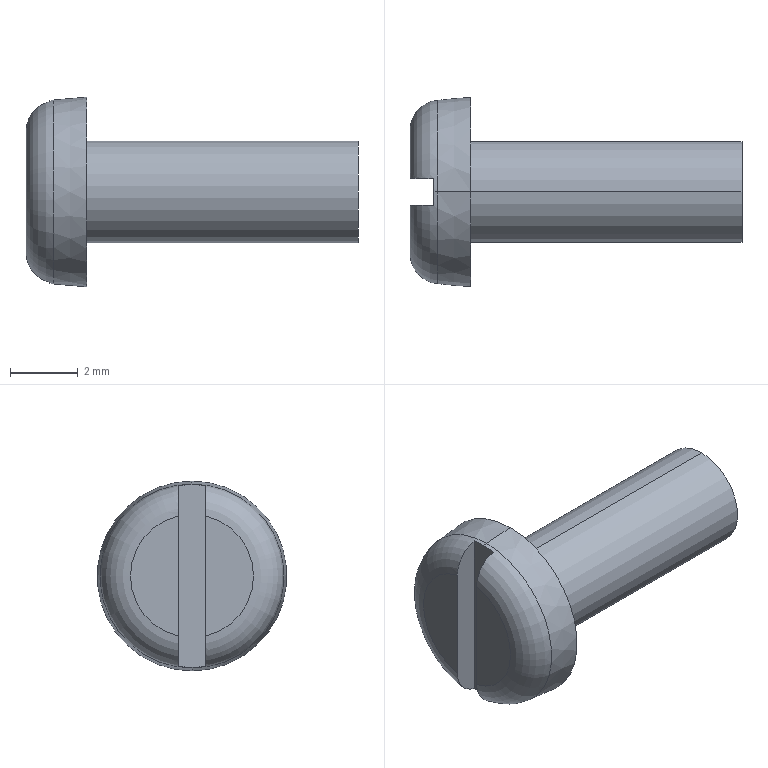Part | SolidWorks | features Fillet 2, Attribute 1, Cut 1, LPattern 1, RevCut 1, Revolution 1 | 1 solid | 13 faces | box 9.8 x 5.6 x 5.6 mm | volume 93.48 mm3 | plane 7 | torus 2 | cone 2 | cylinder 2 | commonest cylinder face diameters 3 x2
STEP:
#1=CARTESIAN_POINT('',(0.8216,0.,-2.714));
#2=VERTEX_POINT('',#1);
#3=CARTESIAN_POINT('',(0.8216,0.,2.714));
#4=VERTEX_POINT('',#3);
#5=CARTESIAN_POINT('',(0.8216,0.,0.));
#6=DIRECTION('',(1.,0.,0.));
#7=DIRECTION('',(0.,0.,1.));
#8=AXIS2_PLACEMENT_3D('',#5,#6,#7);
#9=CIRCLE('',#8,2.714);
#10=EDGE_CURVE('',#2,#4,#9,.T.);
#11=ORIENTED_EDGE('',*,*,#10,.F.);
#12=CARTESIAN_POINT('',(0.7,0.,-2.695));
#13=VERTEX_POINT('',#12);
#14=CARTESIAN_POINT('',(0.9,0.,-1.818));
#15=DIRECTION('',(0.,1.,0.));
#16=DIRECTION('',(0.,0.,1.));
#17=AXIS2_PLACEMENT_3D('',#14,#15,#16);
#18=CIRCLE('',#17,0.9);
#19=EDGE_CURVE('',#2,#13,#18,.T.);
#20=ORIENTED_EDGE('',*,*,#19,.T.);
#21=CARTESIAN_POINT('',(0.7,0.4,-2.665));
#22=VERTEX_POINT('',#21);
#23=CARTESIAN_POINT('',(0.7,0.,0.));
#24=DIRECTION('',(1.,0.,0.));
#25=DIRECTION('',(0.,0.,1.));
#26=AXIS2_PLACEMENT_3D('',#23,#24,#25);
#27=CIRCLE('',#26,2.695);
#28=EDGE_CURVE('',#13,#22,#27,.T.);
#29=ORIENTED_EDGE('',*,*,#28,.T.);
#30=CARTESIAN_POINT('',(0.,0.4,-1.773));
#31=VERTEX_POINT('',#30);
#32=CARTESIAN_POINT('',(0.,0.4,-1.773));
#33=CARTESIAN_POINT('',(0.,0.4,-1.977));
#34=CARTESIAN_POINT('',(0.06786,0.4,-2.18));
#35=CARTESIAN_POINT('',(0.3198,0.4,-2.504));
#36=CARTESIAN_POINT('',(0.5021,0.4,-2.62));
#37=CARTESIAN_POINT('',(0.7,0.4,-2.665));
#38=B_SPLINE_CURVE_WITH_KNOTS('',3,(#32,#33,#34,#35,#36,#37),.UNSPECIFIED.,.F.,.F.,(4,2,4),(0.004973,0.005582,0.006191),.UNSPECIFIED.);
#39=EDGE_CURVE('',#31,#22,#38,.T.);
#40=ORIENTED_EDGE('',*,*,#39,.F.);
#41=CARTESIAN_POINT('',(0.,0.4,1.773));
#42=VERTEX_POINT('',#41);
#43=CARTESIAN_POINT('',(0.,0.,0.));
#44=DIRECTION('',(-1.,0.,0.));
#45=DIRECTION('',(0.,0.,1.));
#46=AXIS2_PLACEMENT_3D('',#43,#44,#45);
#47=CIRCLE('',#46,1.818);
#48=EDGE_CURVE('',#42,#31,#47,.T.);
#49=ORIENTED_EDGE('',*,*,#48,.F.);
#50=CARTESIAN_POINT('',(0.7,0.4,2.665));
#51=VERTEX_POINT('',#50);
#52=CARTESIAN_POINT('',(0.7,0.4,2.665));
#53=CARTESIAN_POINT('',(0.4997,0.4,2.619));
#54=CARTESIAN_POINT('',(0.3202,0.4,2.504));
#55=CARTESIAN_POINT('',(0.06789,0.4,2.18));
#56=CARTESIAN_POINT('',(0.,0.4,1.978));
#57=CARTESIAN_POINT('',(0.,0.4,1.773));
#58=B_SPLINE_CURVE_WITH_KNOTS('',3,(#52,#53,#54,#55,#56,#57),.UNSPECIFIED.,.F.,.F.,(4,2,4),(0.00365,0.004259,0.004869),.UNSPECIFIED.);
#59=EDGE_CURVE('',#51,#42,#58,.T.);
#60=ORIENTED_EDGE('',*,*,#59,.F.);
#61=CARTESIAN_POINT('',(0.7,0.,2.695));
#62=VERTEX_POINT('',#61);
#63=CARTESIAN_POINT('',(0.7,0.,0.));
#64=DIRECTION('',(1.,0.,0.));
#65=DIRECTION('',(0.,0.,1.));
#66=AXIS2_PLACEMENT_3D('',#63,#64,#65);
#67=CIRCLE('',#66,2.695);
#68=EDGE_CURVE('',#51,#62,#67,.T.);
#69=ORIENTED_EDGE('',*,*,#68,.T.);
#70=CARTESIAN_POINT('',(0.9,0.,1.818));
#71=DIRECTION('',(0.,-1.,0.));
#72=DIRECTION('',(0.,0.,-1.));
#73=AXIS2_PLACEMENT_3D('',#70,#71,#72);
#74=CIRCLE('',#73,0.9);
#75=EDGE_CURVE('',#4,#62,#74,.T.);
#76=ORIENTED_EDGE('',*,*,#75,.F.);
#77=EDGE_LOOP('',(#11,#20,#29,#40,#49,#60,#69,#76));
#78=FACE_OUTER_BOUND('',#77,.T.);
#79=CARTESIAN_POINT('',(0.9,0.,0.));
#80=DIRECTION('',(-1.,0.,0.));
#81=DIRECTION('',(0.,0.,1.));
#82=AXIS2_PLACEMENT_3D('',#79,#80,#81);
#83=TOROIDAL_SURFACE('',#82,1.818,0.9);
#84=ADVANCED_FACE('',(#78),#83,.T.);
#85=ORIENTED_EDGE('',*,*,#10,.T.);
#86=CARTESIAN_POINT('',(1.8,0.,2.8));
#87=VERTEX_POINT('',#86);
#88=CARTESIAN_POINT('',(0.,0.,2.643));
#89=DIRECTION('',(0.9962,0.,0.08716));
#90=VECTOR('',#89,1000.);
#91=LINE('',#88,#90);
#92=EDGE_CURVE('',#4,#87,#91,.T.);
#93=ORIENTED_EDGE('',*,*,#92,.T.);
#94=CARTESIAN_POINT('',(1.8,0.,-2.8));
#95=VERTEX_POINT('',#94);
#96=CARTESIAN_POINT('',(1.8,0.,0.));
#97=DIRECTION('',(-1.,0.,0.));
#98=DIRECTION('',(0.,0.,1.));
#99=AXIS2_PLACEMENT_3D('',#96,#97,#98);
#100=CIRCLE('',#99,2.8);
#101=EDGE_CURVE('',#87,#95,#100,.T.);
#102=ORIENTED_EDGE('',*,*,#101,.T.);
#103=CARTESIAN_POINT('',(0.,0.,-2.643));
#104=DIRECTION('',(0.9962,0.,-0.08716));
#105=VECTOR('',#104,1000.);
#106=LINE('',#103,#105);
#107=EDGE_CURVE('',#2,#95,#106,.T.);
#108=ORIENTED_EDGE('',*,*,#107,.F.);
#109=EDGE_LOOP('',(#85,#93,#102,#108));
#110=FACE_OUTER_BOUND('',#109,.T.);
#111=CARTESIAN_POINT('',(0.,0.,0.));
#112=DIRECTION('',(1.,0.,0.));
#113=DIRECTION('',(0.,0.,-1.));
#114=AXIS2_PLACEMENT_3D('',#111,#112,#113);
#115=CONICAL_SURFACE('',#114,2.643,0.08727);
#116=ADVANCED_FACE('',(#110),#115,.T.);
#117=CARTESIAN_POINT('',(9.8,0.,1.5));
#118=VERTEX_POINT('',#117);
#119=CARTESIAN_POINT('',(9.8,0.,-1.5));
#120=VERTEX_POINT('',#119);
#121=CARTESIAN_POINT('',(9.8,0.,0.));
#122=DIRECTION('',(-1.,0.,0.));
#123=DIRECTION('',(0.,0.,1.));
#124=AXIS2_PLACEMENT_3D('',#121,#122,#123);
#125=CIRCLE('',#124,1.5);
#126=EDGE_CURVE('',#118,#120,#125,.T.);
#127=ORIENTED_EDGE('',*,*,#126,.T.);
#128=CARTESIAN_POINT('',(1.8,0.,-1.5));
#129=VERTEX_POINT('',#128);
#130=CARTESIAN_POINT('',(-25.4,0.,-1.5));
#131=DIRECTION('',(-1.,0.,0.));
#132=VECTOR('',#131,1000.);
#133=LINE('',#130,#132);
#134=EDGE_CURVE('',#120,#129,#133,.T.);
#135=ORIENTED_EDGE('',*,*,#134,.T.);
#136=CARTESIAN_POINT('',(1.8,0.,1.5));
#137=VERTEX_POINT('',#136);
#138=CARTESIAN_POINT('',(1.8,0.,0.));
#139=DIRECTION('',(-1.,0.,0.));
#140=DIRECTION('',(0.,0.,1.));
#141=AXIS2_PLACEMENT_3D('',#138,#139,#140);
#142=CIRCLE('',#141,1.5);
#143=EDGE_CURVE('',#137,#129,#142,.T.);
#144=ORIENTED_EDGE('',*,*,#143,.F.);
#145=CARTESIAN_POINT('',(-25.4,0.,1.5));
#146=DIRECTION('',(-1.,0.,0.));
#147=VECTOR('',#146,1000.);
#148=LINE('',#145,#147);
#149=EDGE_CURVE('',#118,#137,#148,.T.);
#150=ORIENTED_EDGE('',*,*,#149,.F.);
#151=EDGE_LOOP('',(#127,#135,#144,#150));
#152=FACE_OUTER_BOUND('',#151,.T.);
#153=CARTESIAN_POINT('',(-25.4,0.,0.));
#154=DIRECTION('',(-1.,0.,0.));
#155=DIRECTION('',(0.,0.,1.));
#156=AXIS2_PLACEMENT_3D('',#153,#154,#155);
#157=CYLINDRICAL_SURFACE('',#156,1.5);
#158=ADVANCED_FACE('',(#152),#157,.T.);
#159=CARTESIAN_POINT('',(0.,0.4,2.8));
#160=DIRECTION('',(0.,0.,-1.));
#161=VECTOR('',#160,1000.);
#162=LINE('',#159,#161);
#163=EDGE_CURVE('',#42,#31,#162,.T.);
#164=ORIENTED_EDGE('',*,*,#163,.F.);
#165=ORIENTED_EDGE('',*,*,#48,.T.);
#166=EDGE_LOOP('',(#164,#165));
#167=FACE_OUTER_BOUND('',#166,.T.);
#168=CARTESIAN_POINT('',(0.,0.,0.));
#169=DIRECTION('',(-1.,0.,0.));
#170=DIRECTION('',(0.,0.,1.));
#171=AXIS2_PLACEMENT_3D('',#168,#169,#170);
#172=PLANE('',#171);
#173=ADVANCED_FACE('',(#167),#172,.T.);
#174=ORIENTED_EDGE('',*,*,#134,.F.);
#175=CARTESIAN_POINT('',(9.8,0.,0.));
#176=DIRECTION('',(-1.,0.,0.));
#177=DIRECTION('',(0.,0.,1.));
#178=AXIS2_PLACEMENT_3D('',#175,#176,#177);
#179=CIRCLE('',#178,1.5);
#180=EDGE_CURVE('',#120,#118,#179,.T.);
#181=ORIENTED_EDGE('',*,*,#180,.T.);
#182=ORIENTED_EDGE('',*,*,#149,.T.);
#183=CARTESIAN_POINT('',(1.8,0.,0.));
#184=DIRECTION('',(-1.,0.,0.));
#185=DIRECTION('',(0.,0.,1.));
#186=AXIS2_PLACEMENT_3D('',#183,#184,#185);
#187=CIRCLE('',#186,1.5);
#188=EDGE_CURVE('',#129,#137,#187,.T.);
#189=ORIENTED_EDGE('',*,*,#188,.F.);
#190=EDGE_LOOP('',(#174,#181,#182,#189));
#191=FACE_OUTER_BOUND('',#190,.T.);
#192=CARTESIAN_POINT('',(-25.4,0.,0.));
#193=DIRECTION('',(-1.,0.,0.));
#194=DIRECTION('',(0.,0.,1.));
#195=AXIS2_PLACEMENT_3D('',#192,#193,#194);
#196=CYLINDRICAL_SURFACE('',#195,1.5);
#197=ADVANCED_FACE('',(#191),#196,.T.);
#198=ORIENTED_EDGE('',*,*,#126,.F.);
#199=ORIENTED_EDGE('',*,*,#180,.F.);
#200=EDGE_LOOP('',(#198,#199));
#201=FACE_OUTER_BOUND('',#200,.T.);
#202=CARTESIAN_POINT('',(9.8,1.5,0.));
#203=DIRECTION('',(1.,0.,0.));
#204=DIRECTION('',(0.,0.,-1.));
#205=AXIS2_PLACEMENT_3D('',#202,#203,#204);
#206=PLANE('',#205);
#207=ADVANCED_FACE('',(#201),#206,.T.);
#208=CARTESIAN_POINT('',(0.,-0.4,-1.773));
#209=VERTEX_POINT('',#208);
#210=CARTESIAN_POINT('',(0.,-0.4,1.773));
#211=VERTEX_POINT('',#210);
#212=CARTESIAN_POINT('',(0.,-0.4,-2.8));
#213=DIRECTION('',(0.,0.,1.));
#214=VECTOR('',#213,1000.);
#215=LINE('',#212,#214);
#216=EDGE_CURVE('',#209,#211,#215,.T.);
#217=ORIENTED_EDGE('',*,*,#216,.F.);
#218=CARTESIAN_POINT('',(0.,0.,0.));
#219=DIRECTION('',(-1.,0.,0.));
#220=DIRECTION('',(0.,0.,1.));
#221=AXIS2_PLACEMENT_3D('',#218,#219,#220);
#222=CIRCLE('',#221,1.818);
#223=EDGE_CURVE('',#209,#211,#222,.T.);
#224=ORIENTED_EDGE('',*,*,#223,.T.);
#225=EDGE_LOOP('',(#217,#224));
#226=FACE_OUTER_BOUND('',#225,.T.);
#227=CARTESIAN_POINT('',(0.,0.,0.));
#228=DIRECTION('',(-1.,0.,0.));
#229=DIRECTION('',(0.,0.,1.));
#230=AXIS2_PLACEMENT_3D('',#227,#228,#229);
#231=PLANE('',#230);
#232=ADVANCED_FACE('',(#226),#231,.T.);
#233=ORIENTED_EDGE('',*,*,#92,.F.);
#234=CARTESIAN_POINT('',(0.8216,0.,0.));
#235=DIRECTION('',(1.,0.,0.));
#236=DIRECTION('',(0.,0.,1.));
#237=AXIS2_PLACEMENT_3D('',#234,#235,#236);
#238=CIRCLE('',#237,2.714);
#239=EDGE_CURVE('',#4,#2,#238,.T.);
#240=ORIENTED_EDGE('',*,*,#239,.T.);
#241=ORIENTED_EDGE('',*,*,#107,.T.);
#242=CARTESIAN_POINT('',(1.8,0.,0.));
#243=DIRECTION('',(-1.,0.,0.));
#244=DIRECTION('',(0.,0.,1.));
#245=AXIS2_PLACEMENT_3D('',#242,#243,#244);
#246=CIRCLE('',#245,2.8);
#247=EDGE_CURVE('',#95,#87,#246,.T.);
#248=ORIENTED_EDGE('',*,*,#247,.T.);
#249=EDGE_LOOP('',(#233,#240,#241,#248));
#250=FACE_OUTER_BOUND('',#249,.T.);
#251=CARTESIAN_POINT('',(0.,0.,0.));
#252=DIRECTION('',(1.,0.,0.));
#253=DIRECTION('',(0.,0.,-1.));
#254=AXIS2_PLACEMENT_3D('',#251,#252,#253);
#255=CONICAL_SURFACE('',#254,2.643,0.08727);
#256=ADVANCED_FACE('',(#250),#255,.T.);
#257=ORIENTED_EDGE('',*,*,#247,.F.);
#258=ORIENTED_EDGE('',*,*,#101,.F.);
#259=EDGE_LOOP('',(#257,#258));
#260=FACE_OUTER_BOUND('',#259,.T.);
#261=ORIENTED_EDGE('',*,*,#143,.T.);
#262=ORIENTED_EDGE('',*,*,#188,.T.);
#263=EDGE_LOOP('',(#261,#262));
#264=FACE_BOUND('',#263,.T.);
#265=CARTESIAN_POINT('',(1.8,1.5,0.));
#266=DIRECTION('',(-1.,0.,0.));
#267=DIRECTION('',(0.,0.,1.));
#268=AXIS2_PLACEMENT_3D('',#265,#266,#267);
#269=PLANE('',#268);
#270=ADVANCED_FACE('',(#260,#264),#269,.F.);
#271=ORIENTED_EDGE('',*,*,#19,.F.);
#272=ORIENTED_EDGE('',*,*,#239,.F.);
#273=ORIENTED_EDGE('',*,*,#75,.T.);
#274=CARTESIAN_POINT('',(0.7,-0.4,2.665));
#275=VERTEX_POINT('',#274);
#276=CARTESIAN_POINT('',(0.7,0.,0.));
#277=DIRECTION('',(1.,0.,0.));
#278=DIRECTION('',(0.,0.,1.));
#279=AXIS2_PLACEMENT_3D('',#276,#277,#278);
#280=CIRCLE('',#279,2.695);
#281=EDGE_CURVE('',#62,#275,#280,.T.);
#282=ORIENTED_EDGE('',*,*,#281,.T.);
#283=CARTESIAN_POINT('',(0.,-0.4,1.773));
#284=CARTESIAN_POINT('',(0.,-0.4,1.976));
#285=CARTESIAN_POINT('',(0.06918,-0.4,2.182));
#286=CARTESIAN_POINT('',(0.3188,-0.4,2.502));
#287=CARTESIAN_POINT('',(0.502,-0.4,2.62));
#288=CARTESIAN_POINT('',(0.7,-0.4,2.665));
#289=B_SPLINE_CURVE_WITH_KNOTS('',3,(#283,#284,#285,#286,#287,#288),.UNSPECIFIED.,.F.,.F.,(4,2,4),(0.0008521,0.001461,0.00207),.UNSPECIFIED.);
#290=EDGE_CURVE('',#211,#275,#289,.T.);
#291=ORIENTED_EDGE('',*,*,#290,.F.);
#292=ORIENTED_EDGE('',*,*,#223,.F.);
#293=CARTESIAN_POINT('',(0.7,-0.4,-2.665));
#294=VERTEX_POINT('',#293);
#295=CARTESIAN_POINT('',(0.7,-0.4,-2.665));
#296=CARTESIAN_POINT('',(0.5997,-0.4,-2.642));
#297=CARTESIAN_POINT('',(0.506,-0.4,-2.603));
#298=CARTESIAN_POINT('',(0.3326,-0.4,-2.492));
#299=CARTESIAN_POINT('',(0.2559,-0.4,-2.422));
#300=CARTESIAN_POINT('',(0.06903,-0.4,-2.182));
#301=CARTESIAN_POINT('',(0.,-0.4,-1.976));
#302=CARTESIAN_POINT('',(0.,-0.4,-1.773));
#303=B_SPLINE_CURVE_WITH_KNOTS('',3,(#295,#296,#297,#298,#299,#300,#301,#302),.UNSPECIFIED.,.F.,.F.,(4,2,2,4),(0.005243,0.005548,0.005852,0.00646),.UNSPECIFIED.);
#304=EDGE_CURVE('',#294,#209,#303,.T.);
#305=ORIENTED_EDGE('',*,*,#304,.F.);
#306=CARTESIAN_POINT('',(0.7,0.,0.));
#307=DIRECTION('',(1.,0.,0.));
#308=DIRECTION('',(0.,0.,1.));
#309=AXIS2_PLACEMENT_3D('',#306,#307,#308);
#310=CIRCLE('',#309,2.695);
#311=EDGE_CURVE('',#294,#13,#310,.T.);
#312=ORIENTED_EDGE('',*,*,#311,.T.);
#313=EDGE_LOOP('',(#271,#272,#273,#282,#291,#292,#305,#312));
#314=FACE_OUTER_BOUND('',#313,.T.);
#315=CARTESIAN_POINT('',(0.9,0.,0.));
#316=DIRECTION('',(-1.,0.,0.));
#317=DIRECTION('',(0.,0.,1.));
#318=AXIS2_PLACEMENT_3D('',#315,#316,#317);
#319=TOROIDAL_SURFACE('',#318,1.818,0.9);
#320=ADVANCED_FACE('',(#314),#319,.T.);
#321=ORIENTED_EDGE('',*,*,#39,.T.);
#322=CARTESIAN_POINT('',(0.7,0.4,2.8));
#323=DIRECTION('',(0.,0.,-1.));
#324=VECTOR('',#323,1000.);
#325=LINE('',#322,#324);
#326=EDGE_CURVE('',#51,#22,#325,.T.);
#327=ORIENTED_EDGE('',*,*,#326,.F.);
#328=ORIENTED_EDGE('',*,*,#59,.T.);
#329=ORIENTED_EDGE('',*,*,#163,.T.);
#330=EDGE_LOOP('',(#321,#327,#328,#329));
#331=FACE_OUTER_BOUND('',#330,.T.);
#332=CARTESIAN_POINT('',(0.7,0.4,2.8));
#333=DIRECTION('',(0.,1.,0.));
#334=DIRECTION('',(0.,0.,1.));
#335=AXIS2_PLACEMENT_3D('',#332,#333,#334);
#336=PLANE('',#335);
#337=ADVANCED_FACE('',(#331),#336,.F.);
#338=ORIENTED_EDGE('',*,*,#304,.T.);
#339=ORIENTED_EDGE('',*,*,#216,.T.);
#340=ORIENTED_EDGE('',*,*,#290,.T.);
#341=CARTESIAN_POINT('',(0.7,-0.4,-2.8));
#342=DIRECTION('',(0.,0.,1.));
#343=VECTOR('',#342,1000.);
#344=LINE('',#341,#343);
#345=EDGE_CURVE('',#294,#275,#344,.T.);
#346=ORIENTED_EDGE('',*,*,#345,.F.);
#347=EDGE_LOOP('',(#338,#339,#340,#346));
#348=FACE_OUTER_BOUND('',#347,.T.);
#349=CARTESIAN_POINT('',(0.7,-0.4,-2.8));
#350=DIRECTION('',(0.,-1.,0.));
#351=DIRECTION('',(0.,0.,-1.));
#352=AXIS2_PLACEMENT_3D('',#349,#350,#351);
#353=PLANE('',#352);
#354=ADVANCED_FACE('',(#348),#353,.F.);
#355=ORIENTED_EDGE('',*,*,#345,.T.);
#356=ORIENTED_EDGE('',*,*,#281,.F.);
#357=ORIENTED_EDGE('',*,*,#68,.F.);
#358=ORIENTED_EDGE('',*,*,#326,.T.);
#359=ORIENTED_EDGE('',*,*,#28,.F.);
#360=ORIENTED_EDGE('',*,*,#311,.F.);
#361=EDGE_LOOP('',(#355,#356,#357,#358,#359,#360));
#362=FACE_OUTER_BOUND('',#361,.T.);
#363=CARTESIAN_POINT('',(0.7,0.4,-2.8));
#364=DIRECTION('',(-1.,0.,0.));
#365=DIRECTION('',(0.,0.,1.));
#366=AXIS2_PLACEMENT_3D('',#363,#364,#365);
#367=PLANE('',#366);
#368=ADVANCED_FACE('',(#362),#367,.T.);
#369=CLOSED_SHELL('',(#84,#116,#158,#173,#197,#207,#232,#256,#270,#320,#337,#354,#368));
#370=MANIFOLD_SOLID_BREP('',#369);
#371=CARTESIAN_POINT('',(0.,0.,0.));
#372=DIRECTION('',(0.,0.,1.));
#373=DIRECTION('',(1.,0.,0.));
#374=AXIS2_PLACEMENT_3D('',#371,#372,#373);
#375=(LENGTH_UNIT()NAMED_UNIT(*)SI_UNIT(.MILLI.,.METRE.));
#376=UNCERTAINTY_MEASURE_WITH_UNIT(LENGTH_MEASURE(0.00001),#375,'','');
#377=(NAMED_UNIT(*)PLANE_ANGLE_UNIT()SI_UNIT($,.RADIAN.));
#378=(NAMED_UNIT(*)SI_UNIT($,.STERADIAN.)SOLID_ANGLE_UNIT());
#379=(GEOMETRIC_REPRESENTATION_CONTEXT(3)GLOBAL_UNCERTAINTY_ASSIGNED_CONTEXT((#376))GLOBAL_UNIT_ASSIGNED_CONTEXT((#375,#377,#378))REPRESENTATION_CONTEXT('',''));
#380=ADVANCED_BREP_SHAPE_REPRESENTATION('',(#370,#374),#379);